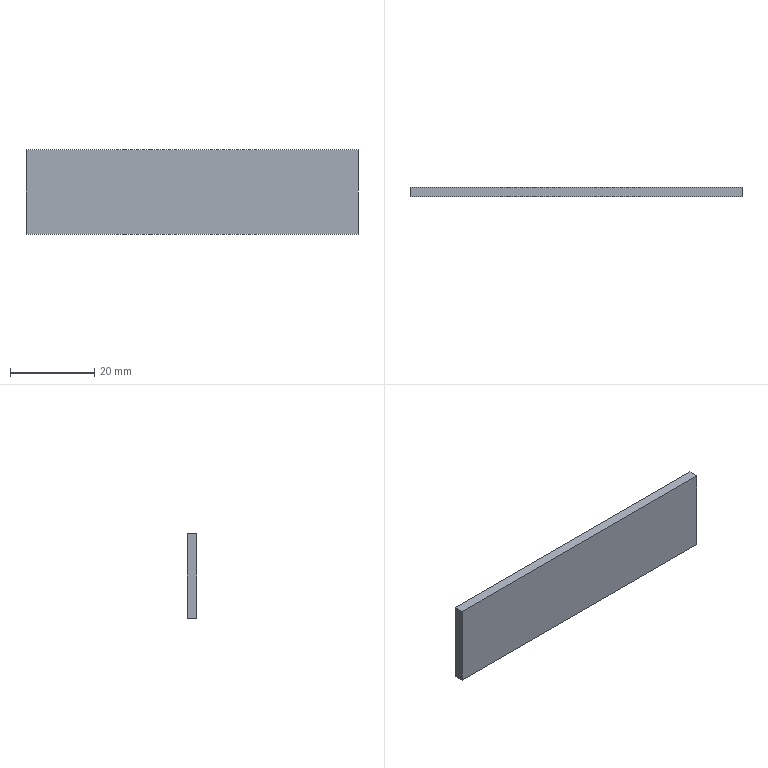Part | SolidWorks | features FlatPattern 1, SMBaseFlange 1, SheetMetal 1 | 1 solid | 6 faces | box 79 x 2.3 x 20 mm | volume 3634 mm3 | plane 6
STEP:
#1=CARTESIAN_POINT('',(0.,0.,0.));
#2=VERTEX_POINT('',#1);
#3=CARTESIAN_POINT('',(0.,0.,20.));
#4=VERTEX_POINT('',#3);
#5=CARTESIAN_POINT('',(0.,0.,0.));
#6=DIRECTION('',(0.,0.,1.));
#7=VECTOR('',#6,1000.);
#8=LINE('',#5,#7);
#9=EDGE_CURVE('',#2,#4,#8,.T.);
#10=ORIENTED_EDGE('',*,*,#9,.F.);
#11=CARTESIAN_POINT('',(0.,-2.3,0.));
#12=VERTEX_POINT('',#11);
#13=CARTESIAN_POINT('',(0.,-2.3,0.));
#14=DIRECTION('',(0.,1.,0.));
#15=VECTOR('',#14,1000.);
#16=LINE('',#13,#15);
#17=EDGE_CURVE('',#12,#2,#16,.T.);
#18=ORIENTED_EDGE('',*,*,#17,.F.);
#19=CARTESIAN_POINT('',(0.,-2.3,20.));
#20=VERTEX_POINT('',#19);
#21=CARTESIAN_POINT('',(0.,-2.3,0.));
#22=DIRECTION('',(0.,0.,1.));
#23=VECTOR('',#22,1000.);
#24=LINE('',#21,#23);
#25=EDGE_CURVE('',#12,#20,#24,.T.);
#26=ORIENTED_EDGE('',*,*,#25,.T.);
#27=CARTESIAN_POINT('',(0.,-2.3,20.));
#28=DIRECTION('',(0.,1.,0.));
#29=VECTOR('',#28,1000.);
#30=LINE('',#27,#29);
#31=EDGE_CURVE('',#20,#4,#30,.T.);
#32=ORIENTED_EDGE('',*,*,#31,.T.);
#33=EDGE_LOOP('',(#10,#18,#26,#32));
#34=FACE_OUTER_BOUND('',#33,.T.);
#35=CARTESIAN_POINT('',(0.,-2.3,0.));
#36=DIRECTION('',(-1.,0.,0.));
#37=DIRECTION('',(0.,0.,1.));
#38=AXIS2_PLACEMENT_3D('',#35,#36,#37);
#39=PLANE('',#38);
#40=ADVANCED_FACE('',(#34),#39,.T.);
#41=CARTESIAN_POINT('',(79.,0.,0.));
#42=VERTEX_POINT('',#41);
#43=CARTESIAN_POINT('',(0.,0.,0.));
#44=DIRECTION('',(-1.,0.,0.));
#45=VECTOR('',#44,1000.);
#46=LINE('',#43,#45);
#47=EDGE_CURVE('',#42,#2,#46,.T.);
#48=ORIENTED_EDGE('',*,*,#47,.F.);
#49=CARTESIAN_POINT('',(79.,-2.3,0.));
#50=VERTEX_POINT('',#49);
#51=CARTESIAN_POINT('',(79.,-2.3,0.));
#52=DIRECTION('',(0.,1.,0.));
#53=VECTOR('',#52,1000.);
#54=LINE('',#51,#53);
#55=EDGE_CURVE('',#50,#42,#54,.T.);
#56=ORIENTED_EDGE('',*,*,#55,.F.);
#57=CARTESIAN_POINT('',(0.,-2.3,0.));
#58=DIRECTION('',(-1.,0.,0.));
#59=VECTOR('',#58,1000.);
#60=LINE('',#57,#59);
#61=EDGE_CURVE('',#50,#12,#60,.T.);
#62=ORIENTED_EDGE('',*,*,#61,.T.);
#63=ORIENTED_EDGE('',*,*,#17,.T.);
#64=EDGE_LOOP('',(#48,#56,#62,#63));
#65=FACE_OUTER_BOUND('',#64,.T.);
#66=CARTESIAN_POINT('',(0.,-2.3,0.));
#67=DIRECTION('',(0.,0.,-1.));
#68=DIRECTION('',(-1.,0.,0.));
#69=AXIS2_PLACEMENT_3D('',#66,#67,#68);
#70=PLANE('',#69);
#71=ADVANCED_FACE('',(#65),#70,.T.);
#72=CARTESIAN_POINT('',(79.,0.,20.));
#73=VERTEX_POINT('',#72);
#74=CARTESIAN_POINT('',(79.,0.,0.));
#75=DIRECTION('',(0.,0.,-1.));
#76=VECTOR('',#75,1000.);
#77=LINE('',#74,#76);
#78=EDGE_CURVE('',#73,#42,#77,.T.);
#79=ORIENTED_EDGE('',*,*,#78,.F.);
#80=CARTESIAN_POINT('',(79.,-2.3,20.));
#81=VERTEX_POINT('',#80);
#82=CARTESIAN_POINT('',(79.,-2.3,20.));
#83=DIRECTION('',(0.,1.,0.));
#84=VECTOR('',#83,1000.);
#85=LINE('',#82,#84);
#86=EDGE_CURVE('',#81,#73,#85,.T.);
#87=ORIENTED_EDGE('',*,*,#86,.F.);
#88=CARTESIAN_POINT('',(79.,-2.3,0.));
#89=DIRECTION('',(0.,0.,-1.));
#90=VECTOR('',#89,1000.);
#91=LINE('',#88,#90);
#92=EDGE_CURVE('',#81,#50,#91,.T.);
#93=ORIENTED_EDGE('',*,*,#92,.T.);
#94=ORIENTED_EDGE('',*,*,#55,.T.);
#95=EDGE_LOOP('',(#79,#87,#93,#94));
#96=FACE_OUTER_BOUND('',#95,.T.);
#97=CARTESIAN_POINT('',(79.,-2.3,0.));
#98=DIRECTION('',(1.,0.,0.));
#99=DIRECTION('',(0.,0.,-1.));
#100=AXIS2_PLACEMENT_3D('',#97,#98,#99);
#101=PLANE('',#100);
#102=ADVANCED_FACE('',(#96),#101,.T.);
#103=CARTESIAN_POINT('',(0.,0.,20.));
#104=DIRECTION('',(1.,0.,0.));
#105=VECTOR('',#104,1000.);
#106=LINE('',#103,#105);
#107=EDGE_CURVE('',#4,#73,#106,.T.);
#108=ORIENTED_EDGE('',*,*,#107,.F.);
#109=ORIENTED_EDGE('',*,*,#31,.F.);
#110=CARTESIAN_POINT('',(0.,-2.3,20.));
#111=DIRECTION('',(1.,0.,0.));
#112=VECTOR('',#111,1000.);
#113=LINE('',#110,#112);
#114=EDGE_CURVE('',#20,#81,#113,.T.);
#115=ORIENTED_EDGE('',*,*,#114,.T.);
#116=ORIENTED_EDGE('',*,*,#86,.T.);
#117=EDGE_LOOP('',(#108,#109,#115,#116));
#118=FACE_OUTER_BOUND('',#117,.T.);
#119=CARTESIAN_POINT('',(0.,-2.3,20.));
#120=DIRECTION('',(0.,0.,1.));
#121=DIRECTION('',(1.,0.,0.));
#122=AXIS2_PLACEMENT_3D('',#119,#120,#121);
#123=PLANE('',#122);
#124=ADVANCED_FACE('',(#118),#123,.T.);
#125=ORIENTED_EDGE('',*,*,#25,.F.);
#126=ORIENTED_EDGE('',*,*,#61,.F.);
#127=ORIENTED_EDGE('',*,*,#92,.F.);
#128=ORIENTED_EDGE('',*,*,#114,.F.);
#129=EDGE_LOOP('',(#125,#126,#127,#128));
#130=FACE_OUTER_BOUND('',#129,.T.);
#131=CARTESIAN_POINT('',(0.,-2.3,0.));
#132=DIRECTION('',(0.,1.,0.));
#133=DIRECTION('',(0.,0.,1.));
#134=AXIS2_PLACEMENT_3D('',#131,#132,#133);
#135=PLANE('',#134);
#136=ADVANCED_FACE('',(#130),#135,.F.);
#137=ORIENTED_EDGE('',*,*,#9,.T.);
#138=ORIENTED_EDGE('',*,*,#107,.T.);
#139=ORIENTED_EDGE('',*,*,#78,.T.);
#140=ORIENTED_EDGE('',*,*,#47,.T.);
#141=EDGE_LOOP('',(#137,#138,#139,#140));
#142=FACE_OUTER_BOUND('',#141,.T.);
#143=CARTESIAN_POINT('',(0.,0.,0.));
#144=DIRECTION('',(0.,1.,0.));
#145=DIRECTION('',(0.,0.,1.));
#146=AXIS2_PLACEMENT_3D('',#143,#144,#145);
#147=PLANE('',#146);
#148=ADVANCED_FACE('',(#142),#147,.T.);
#149=CLOSED_SHELL('',(#40,#71,#102,#124,#136,#148));
#150=MANIFOLD_SOLID_BREP('',#149);
#151=CARTESIAN_POINT('',(0.,0.,0.));
#152=DIRECTION('',(0.,0.,1.));
#153=DIRECTION('',(1.,0.,0.));
#154=AXIS2_PLACEMENT_3D('',#151,#152,#153);
#155=(LENGTH_UNIT()NAMED_UNIT(*)SI_UNIT(.MILLI.,.METRE.));
#156=UNCERTAINTY_MEASURE_WITH_UNIT(LENGTH_MEASURE(0.00001),#155,'','');
#157=(NAMED_UNIT(*)PLANE_ANGLE_UNIT()SI_UNIT($,.RADIAN.));
#158=(NAMED_UNIT(*)SI_UNIT($,.STERADIAN.)SOLID_ANGLE_UNIT());
#159=(GEOMETRIC_REPRESENTATION_CONTEXT(3)GLOBAL_UNCERTAINTY_ASSIGNED_CONTEXT((#156))GLOBAL_UNIT_ASSIGNED_CONTEXT((#155,#157,#158))REPRESENTATION_CONTEXT('',''));
#160=ADVANCED_BREP_SHAPE_REPRESENTATION('',(#150,#154),#159);